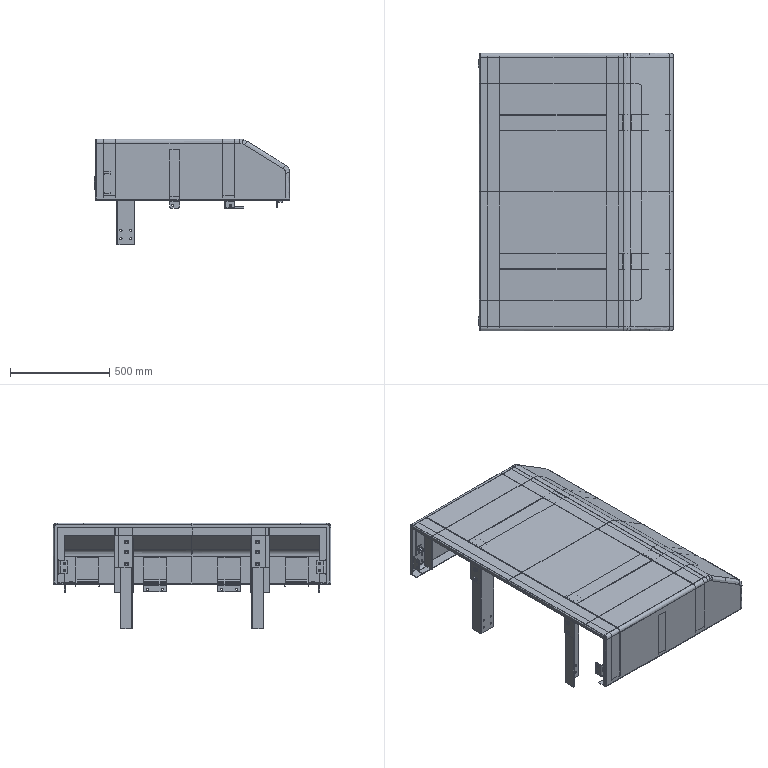Part | NX | features BREP 71 | 71 solids | 1620 faces | box 983.421 x 1400 x 533.004 mm | volume 8293382 mm3 | plane 930 | cylinder 478 | cone 144 | spline 68 | commonest cylinder face diameters 11 x156 10 x48 13 x48 8 x32 9 x28 20 x28